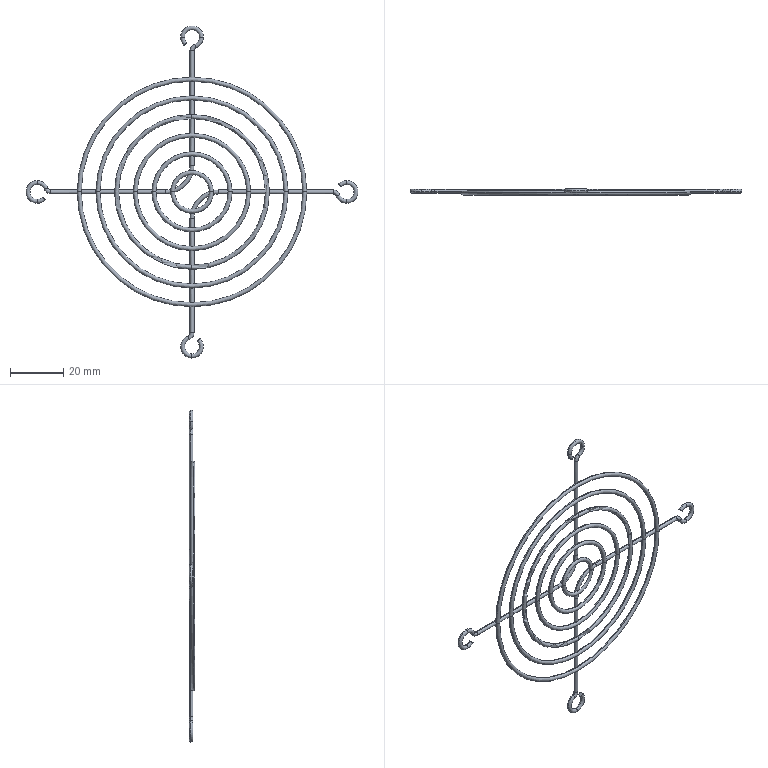Part | STEP file | 82 fan grille | 1 solid | 110 faces | box 124.466 x 2.25 x 124.466 mm | volume 2127 mm3 | torus 76 | cylinder 28 | plane 4 | spline 2 | commonest cylinder face diameters 1.5 x28